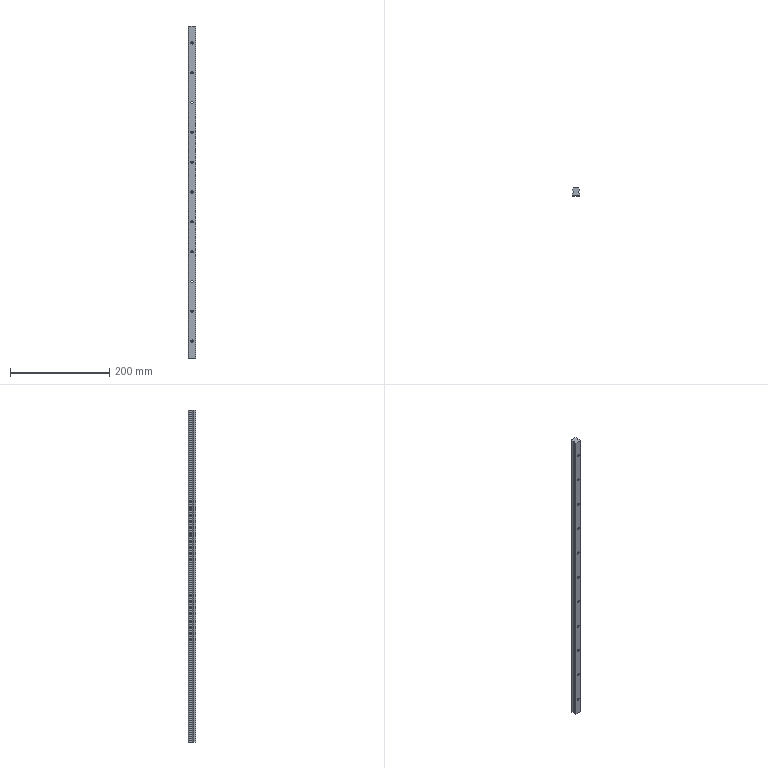Part | STEP file | HGH15 guide rail 2 (HGH15 rail) | 1 solid | 79 faces | box 15 x 15 x 668 mm | volume 127557 mm3 | cylinder 50 | plane 29 | commonest cylinder face diameters 4.5 x22 7.5 x22 0.8 x6